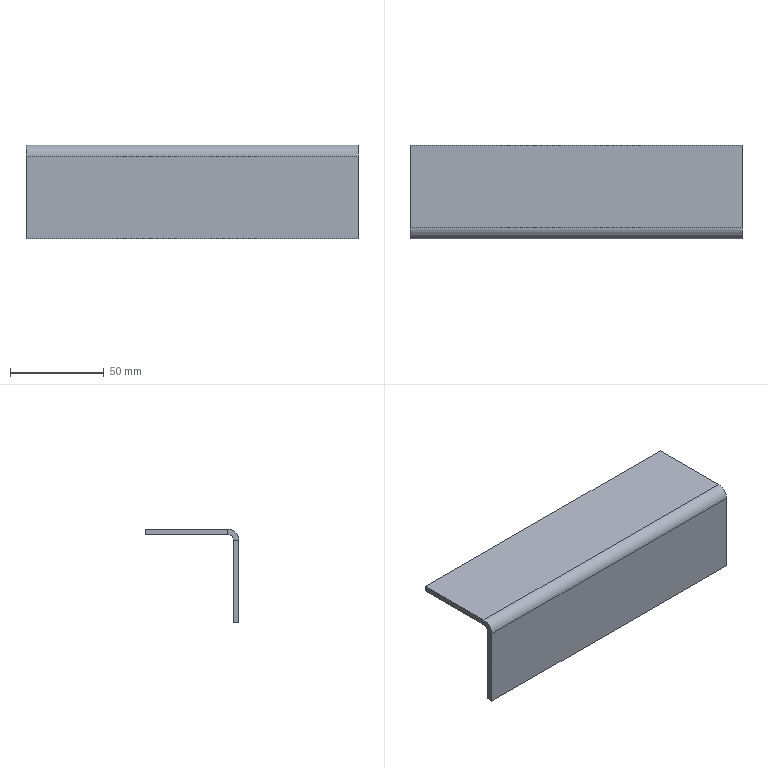Part | SolidWorks | features FlatPattern 1, SMBaseFlange 1, SheetMetal 1 | 1 solid | 14 faces | box 177 x 50 x 50 mm | volume 50481 mm3 | plane 12 | cylinder 2 | commonest cylinder face diameters 6 x1 12 x1
STEP:
#1=CARTESIAN_POINT('',(177.,6.,0.));
#2=VERTEX_POINT('',#1);
#3=CARTESIAN_POINT('',(177.,6.,-3.));
#4=VERTEX_POINT('',#3);
#5=CARTESIAN_POINT('',(177.,6.,0.));
#6=DIRECTION('',(0.,0.,-1.));
#7=VECTOR('',#6,1000.);
#8=LINE('',#5,#7);
#9=EDGE_CURVE('',#2,#4,#8,.T.);
#10=ORIENTED_EDGE('',*,*,#9,.F.);
#11=CARTESIAN_POINT('',(177.,0.,-6.));
#12=VERTEX_POINT('',#11);
#13=CARTESIAN_POINT('',(177.,6.,-6.));
#14=DIRECTION('',(-1.,0.,0.));
#15=DIRECTION('',(0.,0.,-1.));
#16=AXIS2_PLACEMENT_3D('',#13,#14,#15);
#17=CIRCLE('',#16,6.);
#18=EDGE_CURVE('',#12,#2,#17,.T.);
#19=ORIENTED_EDGE('',*,*,#18,.F.);
#20=CARTESIAN_POINT('',(177.,3.,-6.));
#21=VERTEX_POINT('',#20);
#22=CARTESIAN_POINT('',(177.,3.,-6.));
#23=DIRECTION('',(0.,-1.,0.));
#24=VECTOR('',#23,1000.);
#25=LINE('',#22,#24);
#26=EDGE_CURVE('',#21,#12,#25,.T.);
#27=ORIENTED_EDGE('',*,*,#26,.F.);
#28=CARTESIAN_POINT('',(177.,6.,-6.));
#29=DIRECTION('',(-1.,0.,0.));
#30=DIRECTION('',(0.,0.,-1.));
#31=AXIS2_PLACEMENT_3D('',#28,#29,#30);
#32=CIRCLE('',#31,3.);
#33=EDGE_CURVE('',#21,#4,#32,.T.);
#34=ORIENTED_EDGE('',*,*,#33,.T.);
#35=EDGE_LOOP('',(#10,#19,#27,#34));
#36=FACE_OUTER_BOUND('',#35,.T.);
#37=CARTESIAN_POINT('',(177.,6.,0.));
#38=DIRECTION('',(1.,0.,0.));
#39=DIRECTION('',(0.,0.,-1.));
#40=AXIS2_PLACEMENT_3D('',#37,#38,#39);
#41=PLANE('',#40);
#42=ADVANCED_FACE('',(#36),#41,.T.);
#43=CARTESIAN_POINT('',(177.,50.,0.));
#44=VERTEX_POINT('',#43);
#45=CARTESIAN_POINT('',(177.,0.,0.));
#46=DIRECTION('',(0.,1.,0.));
#47=VECTOR('',#46,1000.);
#48=LINE('',#45,#47);
#49=EDGE_CURVE('',#2,#44,#48,.T.);
#50=ORIENTED_EDGE('',*,*,#49,.F.);
#51=ORIENTED_EDGE('',*,*,#9,.T.);
#52=CARTESIAN_POINT('',(177.,50.,-3.));
#53=VERTEX_POINT('',#52);
#54=CARTESIAN_POINT('',(177.,0.,-3.));
#55=DIRECTION('',(0.,1.,0.));
#56=VECTOR('',#55,1000.);
#57=LINE('',#54,#56);
#58=EDGE_CURVE('',#4,#53,#57,.T.);
#59=ORIENTED_EDGE('',*,*,#58,.T.);
#60=CARTESIAN_POINT('',(177.,50.,0.));
#61=DIRECTION('',(0.,0.,-1.));
#62=VECTOR('',#61,1000.);
#63=LINE('',#60,#62);
#64=EDGE_CURVE('',#44,#53,#63,.T.);
#65=ORIENTED_EDGE('',*,*,#64,.F.);
#66=EDGE_LOOP('',(#50,#51,#59,#65));
#67=FACE_OUTER_BOUND('',#66,.T.);
#68=CARTESIAN_POINT('',(177.,3.,-6.));
#69=DIRECTION('',(1.,0.,0.));
#70=DIRECTION('',(0.,0.,-1.));
#71=AXIS2_PLACEMENT_3D('',#68,#69,#70);
#72=PLANE('',#71);
#73=ADVANCED_FACE('',(#67),#72,.T.);
#74=CARTESIAN_POINT('',(0.,0.,-6.));
#75=VERTEX_POINT('',#74);
#76=CARTESIAN_POINT('',(0.,3.,-6.));
#77=VERTEX_POINT('',#76);
#78=CARTESIAN_POINT('',(0.,0.,-6.));
#79=DIRECTION('',(0.,1.,0.));
#80=VECTOR('',#79,1000.);
#81=LINE('',#78,#80);
#82=EDGE_CURVE('',#75,#77,#81,.T.);
#83=ORIENTED_EDGE('',*,*,#82,.F.);
#84=CARTESIAN_POINT('',(0.,6.,0.));
#85=VERTEX_POINT('',#84);
#86=CARTESIAN_POINT('',(0.,6.,-6.));
#87=DIRECTION('',(-1.,0.,0.));
#88=DIRECTION('',(0.,0.,-1.));
#89=AXIS2_PLACEMENT_3D('',#86,#87,#88);
#90=CIRCLE('',#89,6.);
#91=EDGE_CURVE('',#75,#85,#90,.T.);
#92=ORIENTED_EDGE('',*,*,#91,.T.);
#93=CARTESIAN_POINT('',(0.,6.,-3.));
#94=VERTEX_POINT('',#93);
#95=CARTESIAN_POINT('',(0.,6.,-3.));
#96=DIRECTION('',(0.,0.,1.));
#97=VECTOR('',#96,1000.);
#98=LINE('',#95,#97);
#99=EDGE_CURVE('',#94,#85,#98,.T.);
#100=ORIENTED_EDGE('',*,*,#99,.F.);
#101=CARTESIAN_POINT('',(0.,6.,-6.));
#102=DIRECTION('',(-1.,0.,0.));
#103=DIRECTION('',(0.,0.,-1.));
#104=AXIS2_PLACEMENT_3D('',#101,#102,#103);
#105=CIRCLE('',#104,3.);
#106=EDGE_CURVE('',#77,#94,#105,.T.);
#107=ORIENTED_EDGE('',*,*,#106,.F.);
#108=EDGE_LOOP('',(#83,#92,#100,#107));
#109=FACE_OUTER_BOUND('',#108,.T.);
#110=CARTESIAN_POINT('',(0.,0.,-6.));
#111=DIRECTION('',(-1.,0.,0.));
#112=DIRECTION('',(0.,0.,1.));
#113=AXIS2_PLACEMENT_3D('',#110,#111,#112);
#114=PLANE('',#113);
#115=ADVANCED_FACE('',(#109),#114,.T.);
#116=CARTESIAN_POINT('',(0.,0.,-50.));
#117=VERTEX_POINT('',#116);
#118=CARTESIAN_POINT('',(0.,0.,0.));
#119=DIRECTION('',(0.,0.,1.));
#120=VECTOR('',#119,1000.);
#121=LINE('',#118,#120);
#122=EDGE_CURVE('',#117,#75,#121,.T.);
#123=ORIENTED_EDGE('',*,*,#122,.T.);
#124=ORIENTED_EDGE('',*,*,#82,.T.);
#125=CARTESIAN_POINT('',(0.,3.,-50.));
#126=VERTEX_POINT('',#125);
#127=CARTESIAN_POINT('',(0.,3.,0.));
#128=DIRECTION('',(0.,0.,1.));
#129=VECTOR('',#128,1000.);
#130=LINE('',#127,#129);
#131=EDGE_CURVE('',#126,#77,#130,.T.);
#132=ORIENTED_EDGE('',*,*,#131,.F.);
#133=CARTESIAN_POINT('',(0.,3.,-50.));
#134=DIRECTION('',(0.,-1.,0.));
#135=VECTOR('',#134,1000.);
#136=LINE('',#133,#135);
#137=EDGE_CURVE('',#126,#117,#136,.T.);
#138=ORIENTED_EDGE('',*,*,#137,.T.);
#139=EDGE_LOOP('',(#123,#124,#132,#138));
#140=FACE_OUTER_BOUND('',#139,.T.);
#141=CARTESIAN_POINT('',(0.,6.,-3.));
#142=DIRECTION('',(-1.,0.,0.));
#143=DIRECTION('',(0.,0.,1.));
#144=AXIS2_PLACEMENT_3D('',#141,#142,#143);
#145=PLANE('',#144);
#146=ADVANCED_FACE('',(#140),#145,.T.);
#147=CARTESIAN_POINT('',(0.,50.,-3.));
#148=VERTEX_POINT('',#147);
#149=CARTESIAN_POINT('',(0.,0.,-3.));
#150=DIRECTION('',(0.,1.,0.));
#151=VECTOR('',#150,1000.);
#152=LINE('',#149,#151);
#153=EDGE_CURVE('',#94,#148,#152,.T.);
#154=ORIENTED_EDGE('',*,*,#153,.T.);
#155=CARTESIAN_POINT('',(177.,50.,-3.));
#156=DIRECTION('',(-1.,0.,0.));
#157=VECTOR('',#156,1000.);
#158=LINE('',#155,#157);
#159=EDGE_CURVE('',#53,#148,#158,.T.);
#160=ORIENTED_EDGE('',*,*,#159,.F.);
#161=ORIENTED_EDGE('',*,*,#58,.F.);
#162=CARTESIAN_POINT('',(177.,6.,-3.));
#163=DIRECTION('',(-1.,0.,0.));
#164=VECTOR('',#163,1000.);
#165=LINE('',#162,#164);
#166=EDGE_CURVE('',#4,#94,#165,.T.);
#167=ORIENTED_EDGE('',*,*,#166,.T.);
#168=EDGE_LOOP('',(#154,#160,#161,#167));
#169=FACE_OUTER_BOUND('',#168,.T.);
#170=CARTESIAN_POINT('',(177.,0.,-3.));
#171=DIRECTION('',(0.,0.,1.));
#172=DIRECTION('',(1.,0.,0.));
#173=AXIS2_PLACEMENT_3D('',#170,#171,#172);
#174=PLANE('',#173);
#175=ADVANCED_FACE('',(#169),#174,.F.);
#176=CARTESIAN_POINT('',(0.,50.,0.));
#177=VERTEX_POINT('',#176);
#178=CARTESIAN_POINT('',(0.,50.,0.));
#179=DIRECTION('',(0.,0.,-1.));
#180=VECTOR('',#179,1000.);
#181=LINE('',#178,#180);
#182=EDGE_CURVE('',#177,#148,#181,.T.);
#183=ORIENTED_EDGE('',*,*,#182,.F.);
#184=CARTESIAN_POINT('',(177.,50.,0.));
#185=DIRECTION('',(-1.,0.,0.));
#186=VECTOR('',#185,1000.);
#187=LINE('',#184,#186);
#188=EDGE_CURVE('',#44,#177,#187,.T.);
#189=ORIENTED_EDGE('',*,*,#188,.F.);
#190=ORIENTED_EDGE('',*,*,#64,.T.);
#191=ORIENTED_EDGE('',*,*,#159,.T.);
#192=EDGE_LOOP('',(#183,#189,#190,#191));
#193=FACE_OUTER_BOUND('',#192,.T.);
#194=CARTESIAN_POINT('',(177.,50.,0.));
#195=DIRECTION('',(0.,1.,0.));
#196=DIRECTION('',(0.,0.,1.));
#197=AXIS2_PLACEMENT_3D('',#194,#195,#196);
#198=PLANE('',#197);
#199=ADVANCED_FACE('',(#193),#198,.T.);
#200=CARTESIAN_POINT('',(0.,0.,0.));
#201=DIRECTION('',(0.,1.,0.));
#202=VECTOR('',#201,1000.);
#203=LINE('',#200,#202);
#204=EDGE_CURVE('',#85,#177,#203,.T.);
#205=ORIENTED_EDGE('',*,*,#204,.F.);
#206=CARTESIAN_POINT('',(177.,6.,0.));
#207=DIRECTION('',(-1.,0.,0.));
#208=VECTOR('',#207,1000.);
#209=LINE('',#206,#208);
#210=EDGE_CURVE('',#2,#85,#209,.T.);
#211=ORIENTED_EDGE('',*,*,#210,.F.);
#212=ORIENTED_EDGE('',*,*,#49,.T.);
#213=ORIENTED_EDGE('',*,*,#188,.T.);
#214=EDGE_LOOP('',(#205,#211,#212,#213));
#215=FACE_OUTER_BOUND('',#214,.T.);
#216=CARTESIAN_POINT('',(177.,0.,0.));
#217=DIRECTION('',(0.,0.,1.));
#218=DIRECTION('',(1.,0.,0.));
#219=AXIS2_PLACEMENT_3D('',#216,#217,#218);
#220=PLANE('',#219);
#221=ADVANCED_FACE('',(#215),#220,.T.);
#222=ORIENTED_EDGE('',*,*,#91,.F.);
#223=CARTESIAN_POINT('',(177.,0.,-6.));
#224=DIRECTION('',(-1.,0.,0.));
#225=VECTOR('',#224,1000.);
#226=LINE('',#223,#225);
#227=EDGE_CURVE('',#12,#75,#226,.T.);
#228=ORIENTED_EDGE('',*,*,#227,.F.);
#229=ORIENTED_EDGE('',*,*,#18,.T.);
#230=ORIENTED_EDGE('',*,*,#210,.T.);
#231=EDGE_LOOP('',(#222,#228,#229,#230));
#232=FACE_OUTER_BOUND('',#231,.T.);
#233=CARTESIAN_POINT('',(177.,6.,-6.));
#234=DIRECTION('',(-1.,0.,0.));
#235=DIRECTION('',(0.,0.,1.));
#236=AXIS2_PLACEMENT_3D('',#233,#234,#235);
#237=CYLINDRICAL_SURFACE('',#236,6.);
#238=ADVANCED_FACE('',(#232),#237,.T.);
#239=ORIENTED_EDGE('',*,*,#122,.F.);
#240=CARTESIAN_POINT('',(177.,0.,-50.));
#241=VERTEX_POINT('',#240);
#242=CARTESIAN_POINT('',(177.,0.,-50.));
#243=DIRECTION('',(-1.,0.,0.));
#244=VECTOR('',#243,1000.);
#245=LINE('',#242,#244);
#246=EDGE_CURVE('',#241,#117,#245,.T.);
#247=ORIENTED_EDGE('',*,*,#246,.F.);
#248=CARTESIAN_POINT('',(177.,0.,0.));
#249=DIRECTION('',(0.,0.,1.));
#250=VECTOR('',#249,1000.);
#251=LINE('',#248,#250);
#252=EDGE_CURVE('',#241,#12,#251,.T.);
#253=ORIENTED_EDGE('',*,*,#252,.T.);
#254=ORIENTED_EDGE('',*,*,#227,.T.);
#255=EDGE_LOOP('',(#239,#247,#253,#254));
#256=FACE_OUTER_BOUND('',#255,.T.);
#257=CARTESIAN_POINT('',(177.,0.,0.));
#258=DIRECTION('',(0.,-1.,0.));
#259=DIRECTION('',(0.,0.,-1.));
#260=AXIS2_PLACEMENT_3D('',#257,#258,#259);
#261=PLANE('',#260);
#262=ADVANCED_FACE('',(#256),#261,.T.);
#263=ORIENTED_EDGE('',*,*,#137,.F.);
#264=CARTESIAN_POINT('',(177.,3.,-50.));
#265=VERTEX_POINT('',#264);
#266=CARTESIAN_POINT('',(177.,3.,-50.));
#267=DIRECTION('',(-1.,0.,0.));
#268=VECTOR('',#267,1000.);
#269=LINE('',#266,#268);
#270=EDGE_CURVE('',#265,#126,#269,.T.);
#271=ORIENTED_EDGE('',*,*,#270,.F.);
#272=CARTESIAN_POINT('',(177.,3.,-50.));
#273=DIRECTION('',(0.,-1.,0.));
#274=VECTOR('',#273,1000.);
#275=LINE('',#272,#274);
#276=EDGE_CURVE('',#265,#241,#275,.T.);
#277=ORIENTED_EDGE('',*,*,#276,.T.);
#278=ORIENTED_EDGE('',*,*,#246,.T.);
#279=EDGE_LOOP('',(#263,#271,#277,#278));
#280=FACE_OUTER_BOUND('',#279,.T.);
#281=CARTESIAN_POINT('',(177.,3.,-50.));
#282=DIRECTION('',(0.,0.,-1.));
#283=DIRECTION('',(-1.,0.,0.));
#284=AXIS2_PLACEMENT_3D('',#281,#282,#283);
#285=PLANE('',#284);
#286=ADVANCED_FACE('',(#280),#285,.T.);
#287=ORIENTED_EDGE('',*,*,#131,.T.);
#288=CARTESIAN_POINT('',(177.,3.,-6.));
#289=DIRECTION('',(-1.,0.,0.));
#290=VECTOR('',#289,1000.);
#291=LINE('',#288,#290);
#292=EDGE_CURVE('',#21,#77,#291,.T.);
#293=ORIENTED_EDGE('',*,*,#292,.F.);
#294=CARTESIAN_POINT('',(177.,3.,0.));
#295=DIRECTION('',(0.,0.,1.));
#296=VECTOR('',#295,1000.);
#297=LINE('',#294,#296);
#298=EDGE_CURVE('',#265,#21,#297,.T.);
#299=ORIENTED_EDGE('',*,*,#298,.F.);
#300=ORIENTED_EDGE('',*,*,#270,.T.);
#301=EDGE_LOOP('',(#287,#293,#299,#300));
#302=FACE_OUTER_BOUND('',#301,.T.);
#303=CARTESIAN_POINT('',(177.,3.,0.));
#304=DIRECTION('',(0.,-1.,0.));
#305=DIRECTION('',(0.,0.,-1.));
#306=AXIS2_PLACEMENT_3D('',#303,#304,#305);
#307=PLANE('',#306);
#308=ADVANCED_FACE('',(#302),#307,.F.);
#309=ORIENTED_EDGE('',*,*,#106,.T.);
#310=ORIENTED_EDGE('',*,*,#166,.F.);
#311=ORIENTED_EDGE('',*,*,#33,.F.);
#312=ORIENTED_EDGE('',*,*,#292,.T.);
#313=EDGE_LOOP('',(#309,#310,#311,#312));
#314=FACE_OUTER_BOUND('',#313,.T.);
#315=CARTESIAN_POINT('',(177.,6.,-6.));
#316=DIRECTION('',(-1.,0.,0.));
#317=DIRECTION('',(0.,0.,1.));
#318=AXIS2_PLACEMENT_3D('',#315,#316,#317);
#319=CYLINDRICAL_SURFACE('',#318,3.);
#320=ADVANCED_FACE('',(#314),#319,.F.);
#321=ORIENTED_EDGE('',*,*,#298,.T.);
#322=ORIENTED_EDGE('',*,*,#26,.T.);
#323=ORIENTED_EDGE('',*,*,#252,.F.);
#324=ORIENTED_EDGE('',*,*,#276,.F.);
#325=EDGE_LOOP('',(#321,#322,#323,#324));
#326=FACE_OUTER_BOUND('',#325,.T.);
#327=CARTESIAN_POINT('',(177.,6.,-6.));
#328=DIRECTION('',(1.,0.,0.));
#329=DIRECTION('',(0.,0.,-1.));
#330=AXIS2_PLACEMENT_3D('',#327,#328,#329);
#331=PLANE('',#330);
#332=ADVANCED_FACE('',(#326),#331,.T.);
#333=ORIENTED_EDGE('',*,*,#153,.F.);
#334=ORIENTED_EDGE('',*,*,#99,.T.);
#335=ORIENTED_EDGE('',*,*,#204,.T.);
#336=ORIENTED_EDGE('',*,*,#182,.T.);
#337=EDGE_LOOP('',(#333,#334,#335,#336));
#338=FACE_OUTER_BOUND('',#337,.T.);
#339=CARTESIAN_POINT('',(0.,6.,-6.));
#340=DIRECTION('',(1.,0.,0.));
#341=DIRECTION('',(0.,0.,-1.));
#342=AXIS2_PLACEMENT_3D('',#339,#340,#341);
#343=PLANE('',#342);
#344=ADVANCED_FACE('',(#338),#343,.F.);
#345=CLOSED_SHELL('',(#42,#73,#115,#146,#175,#199,#221,#238,#262,#286,#308,#320,#332,#344));
#346=MANIFOLD_SOLID_BREP('',#345);
#347=CARTESIAN_POINT('',(0.,0.,0.));
#348=DIRECTION('',(0.,0.,1.));
#349=DIRECTION('',(1.,0.,0.));
#350=AXIS2_PLACEMENT_3D('',#347,#348,#349);
#351=(LENGTH_UNIT()NAMED_UNIT(*)SI_UNIT(.MILLI.,.METRE.));
#352=UNCERTAINTY_MEASURE_WITH_UNIT(LENGTH_MEASURE(0.00001),#351,'','');
#353=(NAMED_UNIT(*)PLANE_ANGLE_UNIT()SI_UNIT($,.RADIAN.));
#354=(NAMED_UNIT(*)SI_UNIT($,.STERADIAN.)SOLID_ANGLE_UNIT());
#355=(GEOMETRIC_REPRESENTATION_CONTEXT(3)GLOBAL_UNCERTAINTY_ASSIGNED_CONTEXT((#352))GLOBAL_UNIT_ASSIGNED_CONTEXT((#351,#353,#354))REPRESENTATION_CONTEXT('',''));
#356=ADVANCED_BREP_SHAPE_REPRESENTATION('',(#346,#350),#355);